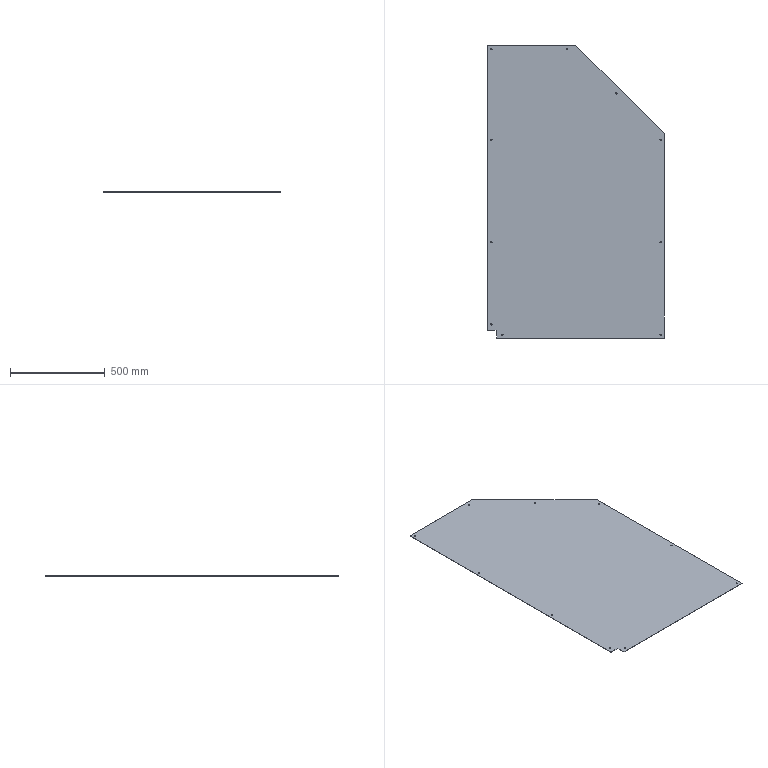Part | SolidWorks | features ICE 5, Fillet 3, HoleWzd 2, Cut 1, FlatPattern 1, SMBaseFlange 1, SheetMetal 1 | 1 solid | 36 faces | box 933 x 1547 x 1.2 mm | volume 1597584 mm3 | cylinder 27 | plane 9 | commonest cylinder face diameters 7 x20 6 x7
STEP:
#1=CARTESIAN_POINT('',(3476.5,-498.,0.));
#2=VERTEX_POINT('',#1);
#3=CARTESIAN_POINT('',(3483.5,-498.,0.));
#4=VERTEX_POINT('',#3);
#5=CARTESIAN_POINT('',(3480.,-498.,0.));
#6=DIRECTION('',(0.,0.,1.));
#7=DIRECTION('',(1.,0.,0.));
#8=AXIS2_PLACEMENT_3D('',#5,#6,#7);
#9=CIRCLE('',#8,3.5);
#10=EDGE_CURVE('',#2,#4,#9,.T.);
#11=ORIENTED_EDGE('',*,*,#10,.F.);
#12=CARTESIAN_POINT('',(3476.5,-498.,1.2));
#13=VERTEX_POINT('',#12);
#14=CARTESIAN_POINT('',(3476.5,-498.,1.2));
#15=DIRECTION('',(0.,0.,1.));
#16=VECTOR('',#15,1000.);
#17=LINE('',#14,#16);
#18=EDGE_CURVE('',#2,#13,#17,.T.);
#19=ORIENTED_EDGE('',*,*,#18,.T.);
#20=CARTESIAN_POINT('',(3483.5,-498.,1.2));
#21=VERTEX_POINT('',#20);
#22=CARTESIAN_POINT('',(3480.,-498.,1.2));
#23=DIRECTION('',(0.,0.,1.));
#24=DIRECTION('',(1.,0.,0.));
#25=AXIS2_PLACEMENT_3D('',#22,#23,#24);
#26=CIRCLE('',#25,3.5);
#27=EDGE_CURVE('',#13,#21,#26,.T.);
#28=ORIENTED_EDGE('',*,*,#27,.T.);
#29=CARTESIAN_POINT('',(3483.5,-498.,1.2));
#30=DIRECTION('',(0.,0.,1.));
#31=VECTOR('',#30,1000.);
#32=LINE('',#29,#31);
#33=EDGE_CURVE('',#4,#21,#32,.T.);
#34=ORIENTED_EDGE('',*,*,#33,.F.);
#35=EDGE_LOOP('',(#11,#19,#28,#34));
#36=FACE_OUTER_BOUND('',#35,.T.);
#37=CARTESIAN_POINT('',(3480.,-498.,1.2));
#38=DIRECTION('',(0.,0.,1.));
#39=DIRECTION('',(1.,0.,0.));
#40=AXIS2_PLACEMENT_3D('',#37,#38,#39);
#41=CYLINDRICAL_SURFACE('',#40,3.5);
#42=ADVANCED_FACE('',(#36),#41,.F.);
#43=CARTESIAN_POINT('',(2583.5,-498.,0.));
#44=VERTEX_POINT('',#43);
#45=CARTESIAN_POINT('',(2590.5,-498.,0.));
#46=VERTEX_POINT('',#45);
#47=CARTESIAN_POINT('',(2587.,-498.,0.));
#48=DIRECTION('',(0.,0.,1.));
#49=DIRECTION('',(1.,0.,0.));
#50=AXIS2_PLACEMENT_3D('',#47,#48,#49);
#51=CIRCLE('',#50,3.5);
#52=EDGE_CURVE('',#44,#46,#51,.T.);
#53=ORIENTED_EDGE('',*,*,#52,.F.);
#54=CARTESIAN_POINT('',(2583.5,-498.,1.2));
#55=VERTEX_POINT('',#54);
#56=CARTESIAN_POINT('',(2583.5,-498.,1.2));
#57=DIRECTION('',(0.,0.,1.));
#58=VECTOR('',#57,1000.);
#59=LINE('',#56,#58);
#60=EDGE_CURVE('',#44,#55,#59,.T.);
#61=ORIENTED_EDGE('',*,*,#60,.T.);
#62=CARTESIAN_POINT('',(2590.5,-498.,1.2));
#63=VERTEX_POINT('',#62);
#64=CARTESIAN_POINT('',(2587.,-498.,1.2));
#65=DIRECTION('',(0.,0.,1.));
#66=DIRECTION('',(1.,0.,0.));
#67=AXIS2_PLACEMENT_3D('',#64,#65,#66);
#68=CIRCLE('',#67,3.5);
#69=EDGE_CURVE('',#55,#63,#68,.T.);
#70=ORIENTED_EDGE('',*,*,#69,.T.);
#71=CARTESIAN_POINT('',(2590.5,-498.,1.2));
#72=DIRECTION('',(0.,0.,1.));
#73=VECTOR('',#72,1000.);
#74=LINE('',#71,#73);
#75=EDGE_CURVE('',#46,#63,#74,.T.);
#76=ORIENTED_EDGE('',*,*,#75,.F.);
#77=EDGE_LOOP('',(#53,#61,#70,#76));
#78=FACE_OUTER_BOUND('',#77,.T.);
#79=CARTESIAN_POINT('',(2587.,-498.,1.2));
#80=DIRECTION('',(0.,0.,1.));
#81=DIRECTION('',(1.,0.,0.));
#82=AXIS2_PLACEMENT_3D('',#79,#80,#81);
#83=CYLINDRICAL_SURFACE('',#82,3.5);
#84=ADVANCED_FACE('',(#78),#83,.F.);
#85=CARTESIAN_POINT('',(2583.5,-20.,0.));
#86=VERTEX_POINT('',#85);
#87=CARTESIAN_POINT('',(2590.5,-20.,0.));
#88=VERTEX_POINT('',#87);
#89=CARTESIAN_POINT('',(2587.,-20.,0.));
#90=DIRECTION('',(0.,0.,1.));
#91=DIRECTION('',(1.,0.,0.));
#92=AXIS2_PLACEMENT_3D('',#89,#90,#91);
#93=CIRCLE('',#92,3.5);
#94=EDGE_CURVE('',#86,#88,#93,.T.);
#95=ORIENTED_EDGE('',*,*,#94,.F.);
#96=CARTESIAN_POINT('',(2583.5,-20.,1.2));
#97=VERTEX_POINT('',#96);
#98=CARTESIAN_POINT('',(2583.5,-20.,1.2));
#99=DIRECTION('',(0.,0.,1.));
#100=VECTOR('',#99,1000.);
#101=LINE('',#98,#100);
#102=EDGE_CURVE('',#86,#97,#101,.T.);
#103=ORIENTED_EDGE('',*,*,#102,.T.);
#104=CARTESIAN_POINT('',(2590.5,-20.,1.2));
#105=VERTEX_POINT('',#104);
#106=CARTESIAN_POINT('',(2587.,-20.,1.2));
#107=DIRECTION('',(0.,0.,1.));
#108=DIRECTION('',(1.,0.,0.));
#109=AXIS2_PLACEMENT_3D('',#106,#107,#108);
#110=CIRCLE('',#109,3.5);
#111=EDGE_CURVE('',#97,#105,#110,.T.);
#112=ORIENTED_EDGE('',*,*,#111,.T.);
#113=CARTESIAN_POINT('',(2590.5,-20.,1.2));
#114=DIRECTION('',(0.,0.,1.));
#115=VECTOR('',#114,1000.);
#116=LINE('',#113,#115);
#117=EDGE_CURVE('',#88,#105,#116,.T.);
#118=ORIENTED_EDGE('',*,*,#117,.F.);
#119=EDGE_LOOP('',(#95,#103,#112,#118));
#120=FACE_OUTER_BOUND('',#119,.T.);
#121=CARTESIAN_POINT('',(2587.,-20.,1.2));
#122=DIRECTION('',(0.,0.,1.));
#123=DIRECTION('',(1.,0.,0.));
#124=AXIS2_PLACEMENT_3D('',#121,#122,#123);
#125=CYLINDRICAL_SURFACE('',#124,3.5);
#126=ADVANCED_FACE('',(#120),#125,.F.);
#127=CARTESIAN_POINT('',(2983.5,-20.,0.));
#128=VERTEX_POINT('',#127);
#129=CARTESIAN_POINT('',(2990.5,-20.,0.));
#130=VERTEX_POINT('',#129);
#131=CARTESIAN_POINT('',(2987.,-20.,0.));
#132=DIRECTION('',(0.,0.,1.));
#133=DIRECTION('',(1.,0.,0.));
#134=AXIS2_PLACEMENT_3D('',#131,#132,#133);
#135=CIRCLE('',#134,3.5);
#136=EDGE_CURVE('',#128,#130,#135,.T.);
#137=ORIENTED_EDGE('',*,*,#136,.F.);
#138=CARTESIAN_POINT('',(2983.5,-20.,1.2));
#139=VERTEX_POINT('',#138);
#140=CARTESIAN_POINT('',(2983.5,-20.,1.2));
#141=DIRECTION('',(0.,0.,1.));
#142=VECTOR('',#141,1000.);
#143=LINE('',#140,#142);
#144=EDGE_CURVE('',#128,#139,#143,.T.);
#145=ORIENTED_EDGE('',*,*,#144,.T.);
#146=CARTESIAN_POINT('',(2990.5,-20.,1.2));
#147=VERTEX_POINT('',#146);
#148=CARTESIAN_POINT('',(2987.,-20.,1.2));
#149=DIRECTION('',(0.,0.,1.));
#150=DIRECTION('',(1.,0.,0.));
#151=AXIS2_PLACEMENT_3D('',#148,#149,#150);
#152=CIRCLE('',#151,3.5);
#153=EDGE_CURVE('',#139,#147,#152,.T.);
#154=ORIENTED_EDGE('',*,*,#153,.T.);
#155=CARTESIAN_POINT('',(2990.5,-20.,1.2));
#156=DIRECTION('',(0.,0.,1.));
#157=VECTOR('',#156,1000.);
#158=LINE('',#155,#157);
#159=EDGE_CURVE('',#130,#147,#158,.T.);
#160=ORIENTED_EDGE('',*,*,#159,.F.);
#161=EDGE_LOOP('',(#137,#145,#154,#160));
#162=FACE_OUTER_BOUND('',#161,.T.);
#163=CARTESIAN_POINT('',(2987.,-20.,1.2));
#164=DIRECTION('',(0.,0.,1.));
#165=DIRECTION('',(1.,0.,0.));
#166=AXIS2_PLACEMENT_3D('',#163,#164,#165);
#167=CYLINDRICAL_SURFACE('',#166,3.5);
#168=ADVANCED_FACE('',(#162),#167,.F.);
#169=CARTESIAN_POINT('',(3476.5,-1039.,0.));
#170=VERTEX_POINT('',#169);
#171=CARTESIAN_POINT('',(3483.5,-1039.,0.));
#172=VERTEX_POINT('',#171);
#173=CARTESIAN_POINT('',(3480.,-1039.,0.));
#174=DIRECTION('',(0.,0.,1.));
#175=DIRECTION('',(1.,0.,0.));
#176=AXIS2_PLACEMENT_3D('',#173,#174,#175);
#177=CIRCLE('',#176,3.5);
#178=EDGE_CURVE('',#170,#172,#177,.T.);
#179=ORIENTED_EDGE('',*,*,#178,.F.);
#180=CARTESIAN_POINT('',(3476.5,-1039.,1.2));
#181=VERTEX_POINT('',#180);
#182=CARTESIAN_POINT('',(3476.5,-1039.,1.2));
#183=DIRECTION('',(0.,0.,1.));
#184=VECTOR('',#183,1000.);
#185=LINE('',#182,#184);
#186=EDGE_CURVE('',#170,#181,#185,.T.);
#187=ORIENTED_EDGE('',*,*,#186,.T.);
#188=CARTESIAN_POINT('',(3483.5,-1039.,1.2));
#189=VERTEX_POINT('',#188);
#190=CARTESIAN_POINT('',(3480.,-1039.,1.2));
#191=DIRECTION('',(0.,0.,1.));
#192=DIRECTION('',(1.,0.,0.));
#193=AXIS2_PLACEMENT_3D('',#190,#191,#192);
#194=CIRCLE('',#193,3.5);
#195=EDGE_CURVE('',#181,#189,#194,.T.);
#196=ORIENTED_EDGE('',*,*,#195,.T.);
#197=CARTESIAN_POINT('',(3483.5,-1039.,1.2));
#198=DIRECTION('',(0.,0.,1.));
#199=VECTOR('',#198,1000.);
#200=LINE('',#197,#199);
#201=EDGE_CURVE('',#172,#189,#200,.T.);
#202=ORIENTED_EDGE('',*,*,#201,.F.);
#203=EDGE_LOOP('',(#179,#187,#196,#202));
#204=FACE_OUTER_BOUND('',#203,.T.);
#205=CARTESIAN_POINT('',(3480.,-1039.,1.2));
#206=DIRECTION('',(0.,0.,1.));
#207=DIRECTION('',(1.,0.,0.));
#208=AXIS2_PLACEMENT_3D('',#205,#206,#207);
#209=CYLINDRICAL_SURFACE('',#208,3.5);
#210=ADVANCED_FACE('',(#204),#209,.F.);
#211=CARTESIAN_POINT('',(3476.5,-1527.,0.));
#212=VERTEX_POINT('',#211);
#213=CARTESIAN_POINT('',(3483.5,-1527.,0.));
#214=VERTEX_POINT('',#213);
#215=CARTESIAN_POINT('',(3480.,-1527.,0.));
#216=DIRECTION('',(0.,0.,1.));
#217=DIRECTION('',(1.,0.,0.));
#218=AXIS2_PLACEMENT_3D('',#215,#216,#217);
#219=CIRCLE('',#218,3.5);
#220=EDGE_CURVE('',#212,#214,#219,.T.);
#221=ORIENTED_EDGE('',*,*,#220,.F.);
#222=CARTESIAN_POINT('',(3476.5,-1527.,1.2));
#223=VERTEX_POINT('',#222);
#224=CARTESIAN_POINT('',(3476.5,-1527.,1.2));
#225=DIRECTION('',(0.,0.,1.));
#226=VECTOR('',#225,1000.);
#227=LINE('',#224,#226);
#228=EDGE_CURVE('',#212,#223,#227,.T.);
#229=ORIENTED_EDGE('',*,*,#228,.T.);
#230=CARTESIAN_POINT('',(3483.5,-1527.,1.2));
#231=VERTEX_POINT('',#230);
#232=CARTESIAN_POINT('',(3480.,-1527.,1.2));
#233=DIRECTION('',(0.,0.,1.));
#234=DIRECTION('',(1.,0.,0.));
#235=AXIS2_PLACEMENT_3D('',#232,#233,#234);
#236=CIRCLE('',#235,3.5);
#237=EDGE_CURVE('',#223,#231,#236,.T.);
#238=ORIENTED_EDGE('',*,*,#237,.T.);
#239=CARTESIAN_POINT('',(3483.5,-1527.,1.2));
#240=DIRECTION('',(0.,0.,1.));
#241=VECTOR('',#240,1000.);
#242=LINE('',#239,#241);
#243=EDGE_CURVE('',#214,#231,#242,.T.);
#244=ORIENTED_EDGE('',*,*,#243,.F.);
#245=EDGE_LOOP('',(#221,#229,#238,#244));
#246=FACE_OUTER_BOUND('',#245,.T.);
#247=CARTESIAN_POINT('',(3480.,-1527.,1.2));
#248=DIRECTION('',(0.,0.,1.));
#249=DIRECTION('',(1.,0.,0.));
#250=AXIS2_PLACEMENT_3D('',#247,#248,#249);
#251=CYLINDRICAL_SURFACE('',#250,3.5);
#252=ADVANCED_FACE('',(#246),#251,.F.);
#253=CARTESIAN_POINT('',(2641.5,-1527.,0.));
#254=VERTEX_POINT('',#253);
#255=CARTESIAN_POINT('',(2648.5,-1527.,0.));
#256=VERTEX_POINT('',#255);
#257=CARTESIAN_POINT('',(2645.,-1527.,0.));
#258=DIRECTION('',(0.,0.,1.));
#259=DIRECTION('',(1.,0.,0.));
#260=AXIS2_PLACEMENT_3D('',#257,#258,#259);
#261=CIRCLE('',#260,3.5);
#262=EDGE_CURVE('',#254,#256,#261,.T.);
#263=ORIENTED_EDGE('',*,*,#262,.F.);
#264=CARTESIAN_POINT('',(2641.5,-1527.,1.2));
#265=VERTEX_POINT('',#264);
#266=CARTESIAN_POINT('',(2641.5,-1527.,1.2));
#267=DIRECTION('',(0.,0.,1.));
#268=VECTOR('',#267,1000.);
#269=LINE('',#266,#268);
#270=EDGE_CURVE('',#254,#265,#269,.T.);
#271=ORIENTED_EDGE('',*,*,#270,.T.);
#272=CARTESIAN_POINT('',(2648.5,-1527.,1.2));
#273=VERTEX_POINT('',#272);
#274=CARTESIAN_POINT('',(2645.,-1527.,1.2));
#275=DIRECTION('',(0.,0.,1.));
#276=DIRECTION('',(1.,0.,0.));
#277=AXIS2_PLACEMENT_3D('',#274,#275,#276);
#278=CIRCLE('',#277,3.5);
#279=EDGE_CURVE('',#265,#273,#278,.T.);
#280=ORIENTED_EDGE('',*,*,#279,.T.);
#281=CARTESIAN_POINT('',(2648.5,-1527.,1.2));
#282=DIRECTION('',(0.,0.,1.));
#283=VECTOR('',#282,1000.);
#284=LINE('',#281,#283);
#285=EDGE_CURVE('',#256,#273,#284,.T.);
#286=ORIENTED_EDGE('',*,*,#285,.F.);
#287=EDGE_LOOP('',(#263,#271,#280,#286));
#288=FACE_OUTER_BOUND('',#287,.T.);
#289=CARTESIAN_POINT('',(2645.,-1527.,1.2));
#290=DIRECTION('',(0.,0.,1.));
#291=DIRECTION('',(1.,0.,0.));
#292=AXIS2_PLACEMENT_3D('',#289,#290,#291);
#293=CYLINDRICAL_SURFACE('',#292,3.5);
#294=ADVANCED_FACE('',(#288),#293,.F.);
#295=CARTESIAN_POINT('',(2583.5,-1472.,0.));
#296=VERTEX_POINT('',#295);
#297=CARTESIAN_POINT('',(2590.5,-1472.,0.));
#298=VERTEX_POINT('',#297);
#299=CARTESIAN_POINT('',(2587.,-1472.,0.));
#300=DIRECTION('',(0.,0.,1.));
#301=DIRECTION('',(1.,0.,0.));
#302=AXIS2_PLACEMENT_3D('',#299,#300,#301);
#303=CIRCLE('',#302,3.5);
#304=EDGE_CURVE('',#296,#298,#303,.T.);
#305=ORIENTED_EDGE('',*,*,#304,.F.);
#306=CARTESIAN_POINT('',(2583.5,-1472.,1.2));
#307=VERTEX_POINT('',#306);
#308=CARTESIAN_POINT('',(2583.5,-1472.,1.2));
#309=DIRECTION('',(0.,0.,1.));
#310=VECTOR('',#309,1000.);
#311=LINE('',#308,#310);
#312=EDGE_CURVE('',#296,#307,#311,.T.);
#313=ORIENTED_EDGE('',*,*,#312,.T.);
#314=CARTESIAN_POINT('',(2590.5,-1472.,1.2));
#315=VERTEX_POINT('',#314);
#316=CARTESIAN_POINT('',(2587.,-1472.,1.2));
#317=DIRECTION('',(0.,0.,1.));
#318=DIRECTION('',(1.,0.,0.));
#319=AXIS2_PLACEMENT_3D('',#316,#317,#318);
#320=CIRCLE('',#319,3.5);
#321=EDGE_CURVE('',#307,#315,#320,.T.);
#322=ORIENTED_EDGE('',*,*,#321,.T.);
#323=CARTESIAN_POINT('',(2590.5,-1472.,1.2));
#324=DIRECTION('',(0.,0.,1.));
#325=VECTOR('',#324,1000.);
#326=LINE('',#323,#325);
#327=EDGE_CURVE('',#298,#315,#326,.T.);
#328=ORIENTED_EDGE('',*,*,#327,.F.);
#329=EDGE_LOOP('',(#305,#313,#322,#328));
#330=FACE_OUTER_BOUND('',#329,.T.);
#331=CARTESIAN_POINT('',(2587.,-1472.,1.2));
#332=DIRECTION('',(0.,0.,1.));
#333=DIRECTION('',(1.,0.,0.));
#334=AXIS2_PLACEMENT_3D('',#331,#332,#333);
#335=CYLINDRICAL_SURFACE('',#334,3.5);
#336=ADVANCED_FACE('',(#330),#335,.F.);
#337=CARTESIAN_POINT('',(3243.074,-253.426,0.));
#338=VERTEX_POINT('',#337);
#339=CARTESIAN_POINT('',(3250.074,-253.426,0.));
#340=VERTEX_POINT('',#339);
#341=CARTESIAN_POINT('',(3246.574,-253.426,0.));
#342=DIRECTION('',(0.,0.,1.));
#343=DIRECTION('',(1.,0.,0.));
#344=AXIS2_PLACEMENT_3D('',#341,#342,#343);
#345=CIRCLE('',#344,3.5);
#346=EDGE_CURVE('',#338,#340,#345,.T.);
#347=ORIENTED_EDGE('',*,*,#346,.F.);
#348=CARTESIAN_POINT('',(3243.074,-253.426,1.2));
#349=VERTEX_POINT('',#348);
#350=CARTESIAN_POINT('',(3243.074,-253.426,1.2));
#351=DIRECTION('',(0.,0.,1.));
#352=VECTOR('',#351,1000.);
#353=LINE('',#350,#352);
#354=EDGE_CURVE('',#338,#349,#353,.T.);
#355=ORIENTED_EDGE('',*,*,#354,.T.);
#356=CARTESIAN_POINT('',(3250.074,-253.426,1.2));
#357=VERTEX_POINT('',#356);
#358=CARTESIAN_POINT('',(3246.574,-253.426,1.2));
#359=DIRECTION('',(0.,0.,1.));
#360=DIRECTION('',(1.,0.,0.));
#361=AXIS2_PLACEMENT_3D('',#358,#359,#360);
#362=CIRCLE('',#361,3.5);
#363=EDGE_CURVE('',#349,#357,#362,.T.);
#364=ORIENTED_EDGE('',*,*,#363,.T.);
#365=CARTESIAN_POINT('',(3250.074,-253.426,1.2));
#366=DIRECTION('',(0.,0.,1.));
#367=VECTOR('',#366,1000.);
#368=LINE('',#365,#367);
#369=EDGE_CURVE('',#340,#357,#368,.T.);
#370=ORIENTED_EDGE('',*,*,#369,.F.);
#371=EDGE_LOOP('',(#347,#355,#364,#370));
#372=FACE_OUTER_BOUND('',#371,.T.);
#373=CARTESIAN_POINT('',(3246.574,-253.426,1.2));
#374=DIRECTION('',(0.,0.,1.));
#375=DIRECTION('',(1.,0.,0.));
#376=AXIS2_PLACEMENT_3D('',#373,#374,#375);
#377=CYLINDRICAL_SURFACE('',#376,3.5);
#378=ADVANCED_FACE('',(#372),#377,.F.);
#379=CARTESIAN_POINT('',(2583.5,-1039.,0.));
#380=VERTEX_POINT('',#379);
#381=CARTESIAN_POINT('',(2590.5,-1039.,0.));
#382=VERTEX_POINT('',#381);
#383=CARTESIAN_POINT('',(2587.,-1039.,0.));
#384=DIRECTION('',(0.,0.,1.));
#385=DIRECTION('',(1.,0.,0.));
#386=AXIS2_PLACEMENT_3D('',#383,#384,#385);
#387=CIRCLE('',#386,3.5);
#388=EDGE_CURVE('',#380,#382,#387,.T.);
#389=ORIENTED_EDGE('',*,*,#388,.F.);
#390=CARTESIAN_POINT('',(2583.5,-1039.,1.2));
#391=VERTEX_POINT('',#390);
#392=CARTESIAN_POINT('',(2583.5,-1039.,1.2));
#393=DIRECTION('',(0.,0.,1.));
#394=VECTOR('',#393,1000.);
#395=LINE('',#392,#394);
#396=EDGE_CURVE('',#380,#391,#395,.T.);
#397=ORIENTED_EDGE('',*,*,#396,.T.);
#398=CARTESIAN_POINT('',(2590.5,-1039.,1.2));
#399=VERTEX_POINT('',#398);
#400=CARTESIAN_POINT('',(2587.,-1039.,1.2));
#401=DIRECTION('',(0.,0.,1.));
#402=DIRECTION('',(1.,0.,0.));
#403=AXIS2_PLACEMENT_3D('',#400,#401,#402);
#404=CIRCLE('',#403,3.5);
#405=EDGE_CURVE('',#391,#399,#404,.T.);
#406=ORIENTED_EDGE('',*,*,#405,.T.);
#407=CARTESIAN_POINT('',(2590.5,-1039.,1.2));
#408=DIRECTION('',(0.,0.,1.));
#409=VECTOR('',#408,1000.);
#410=LINE('',#407,#409);
#411=EDGE_CURVE('',#382,#399,#410,.T.);
#412=ORIENTED_EDGE('',*,*,#411,.F.);
#413=EDGE_LOOP('',(#389,#397,#406,#412));
#414=FACE_OUTER_BOUND('',#413,.T.);
#415=CARTESIAN_POINT('',(2587.,-1039.,1.2));
#416=DIRECTION('',(0.,0.,1.));
#417=DIRECTION('',(1.,0.,0.));
#418=AXIS2_PLACEMENT_3D('',#415,#416,#417);
#419=CYLINDRICAL_SURFACE('',#418,3.5);
#420=ADVANCED_FACE('',(#414),#419,.F.);
#421=CARTESIAN_POINT('',(3497.,-1547.,1.2));
#422=VERTEX_POINT('',#421);
#423=CARTESIAN_POINT('',(2618.,-1547.,1.2));
#424=VERTEX_POINT('',#423);
#425=CARTESIAN_POINT('',(0.,-1547.,1.2));
#426=DIRECTION('',(-1.,0.,0.));
#427=VECTOR('',#426,1000.);
#428=LINE('',#425,#427);
#429=EDGE_CURVE('',#422,#424,#428,.T.);
#430=ORIENTED_EDGE('',*,*,#429,.T.);
#431=CARTESIAN_POINT('',(2618.,-1547.,0.));
#432=VERTEX_POINT('',#431);
#433=CARTESIAN_POINT('',(2618.,-1547.,0.));
#434=DIRECTION('',(0.,0.,-1.));
#435=VECTOR('',#434,1000.);
#436=LINE('',#433,#435);
#437=EDGE_CURVE('',#424,#432,#436,.T.);
#438=ORIENTED_EDGE('',*,*,#437,.T.);
#439=CARTESIAN_POINT('',(3497.,-1547.,0.));
#440=VERTEX_POINT('',#439);
#441=CARTESIAN_POINT('',(0.,-1547.,0.));
#442=DIRECTION('',(-1.,0.,0.));
#443=VECTOR('',#442,1000.);
#444=LINE('',#441,#443);
#445=EDGE_CURVE('',#440,#432,#444,.T.);
#446=ORIENTED_EDGE('',*,*,#445,.F.);
#447=CARTESIAN_POINT('',(3497.,-1547.,1.2));
#448=DIRECTION('',(0.,0.,1.));
#449=VECTOR('',#448,1000.);
#450=LINE('',#447,#449);
#451=EDGE_CURVE('',#440,#422,#450,.T.);
#452=ORIENTED_EDGE('',*,*,#451,.T.);
#453=EDGE_LOOP('',(#430,#438,#446,#452));
#454=FACE_OUTER_BOUND('',#453,.T.);
#455=CARTESIAN_POINT('',(0.,-1547.,1.2));
#456=DIRECTION('',(0.,-1.,0.));
#457=DIRECTION('',(0.,0.,-1.));
#458=AXIS2_PLACEMENT_3D('',#455,#456,#457);
#459=PLANE('',#458);
#460=ADVANCED_FACE('',(#454),#459,.T.);
#461=CARTESIAN_POINT('',(3500.,-469.174,0.));
#462=VERTEX_POINT('',#461);
#463=CARTESIAN_POINT('',(3500.,-1544.,0.));
#464=VERTEX_POINT('',#463);
#465=CARTESIAN_POINT('',(3500.,0.,0.));
#466=DIRECTION('',(0.,-1.,0.));
#467=VECTOR('',#466,1000.);
#468=LINE('',#465,#467);
#469=EDGE_CURVE('',#462,#464,#468,.T.);
#470=ORIENTED_EDGE('',*,*,#469,.F.);
#471=CARTESIAN_POINT('',(3500.,-469.174,1.2));
#472=VERTEX_POINT('',#471);
#473=CARTESIAN_POINT('',(3500.,-469.174,1.2));
#474=DIRECTION('',(0.,0.,1.));
#475=VECTOR('',#474,1000.);
#476=LINE('',#473,#475);
#477=EDGE_CURVE('',#462,#472,#476,.T.);
#478=ORIENTED_EDGE('',*,*,#477,.T.);
#479=CARTESIAN_POINT('',(3500.,-1544.,1.2));
#480=VERTEX_POINT('',#479);
#481=CARTESIAN_POINT('',(3500.,0.,1.2));
#482=DIRECTION('',(0.,-1.,0.));
#483=VECTOR('',#482,1000.);
#484=LINE('',#481,#483);
#485=EDGE_CURVE('',#472,#480,#484,.T.);
#486=ORIENTED_EDGE('',*,*,#485,.T.);
#487=CARTESIAN_POINT('',(3500.,-1544.,1.2));
#488=DIRECTION('',(0.,0.,-1.));
#489=VECTOR('',#488,1000.);
#490=LINE('',#487,#489);
#491=EDGE_CURVE('',#480,#464,#490,.T.);
#492=ORIENTED_EDGE('',*,*,#491,.T.);
#493=EDGE_LOOP('',(#470,#478,#486,#492));
#494=FACE_OUTER_BOUND('',#493,.T.);
#495=CARTESIAN_POINT('',(3500.,0.,1.2));
#496=DIRECTION('',(1.,0.,0.));
#497=DIRECTION('',(0.,0.,-1.));
#498=AXIS2_PLACEMENT_3D('',#495,#496,#497);
#499=PLANE('',#498);
#500=ADVANCED_FACE('',(#494),#499,.T.);
#501=CARTESIAN_POINT('',(2615.,-1544.,1.2));
#502=VERTEX_POINT('',#501);
#503=CARTESIAN_POINT('',(2615.,-1505.,1.2));
#504=VERTEX_POINT('',#503);
#505=CARTESIAN_POINT('',(2615.,-1547.,1.2));
#506=DIRECTION('',(0.,1.,0.));
#507=VECTOR('',#506,1000.);
#508=LINE('',#505,#507);
#509=EDGE_CURVE('',#502,#504,#508,.T.);
#510=ORIENTED_EDGE('',*,*,#509,.T.);
#511=CARTESIAN_POINT('',(2615.,-1505.,0.));
#512=VERTEX_POINT('',#511);
#513=CARTESIAN_POINT('',(2615.,-1505.,0.));
#514=DIRECTION('',(0.,0.,-1.));
#515=VECTOR('',#514,1000.);
#516=LINE('',#513,#515);
#517=EDGE_CURVE('',#504,#512,#516,.T.);
#518=ORIENTED_EDGE('',*,*,#517,.T.);
#519=CARTESIAN_POINT('',(2615.,-1544.,0.));
#520=VERTEX_POINT('',#519);
#521=CARTESIAN_POINT('',(2615.,0.,0.));
#522=DIRECTION('',(0.,1.,0.));
#523=VECTOR('',#522,1000.);
#524=LINE('',#521,#523);
#525=EDGE_CURVE('',#520,#512,#524,.T.);
#526=ORIENTED_EDGE('',*,*,#525,.F.);
#527=CARTESIAN_POINT('',(2615.,-1544.,1.2));
#528=DIRECTION('',(0.,0.,1.));
#529=VECTOR('',#528,1000.);
#530=LINE('',#527,#529);
#531=EDGE_CURVE('',#520,#502,#530,.T.);
#532=ORIENTED_EDGE('',*,*,#531,.T.);
#533=EDGE_LOOP('',(#510,#518,#526,#532));
#534=FACE_OUTER_BOUND('',#533,.T.);
#535=CARTESIAN_POINT('',(2615.,-1547.,-8.8));
#536=DIRECTION('',(1.,0.,0.));
#537=DIRECTION('',(0.,0.,-1.));
#538=AXIS2_PLACEMENT_3D('',#535,#536,#537);
#539=PLANE('',#538);
#540=ADVANCED_FACE('',(#534),#539,.F.);
#541=CARTESIAN_POINT('',(2612.,-1502.,1.2));
#542=VERTEX_POINT('',#541);
#543=CARTESIAN_POINT('',(2570.,-1502.,1.2));
#544=VERTEX_POINT('',#543);
#545=CARTESIAN_POINT('',(885.,-1502.,1.2));
#546=DIRECTION('',(-1.,0.,0.));
#547=VECTOR('',#546,1000.);
#548=LINE('',#545,#547);
#549=EDGE_CURVE('',#542,#544,#548,.T.);
#550=ORIENTED_EDGE('',*,*,#549,.T.);
#551=CARTESIAN_POINT('',(2570.,-1502.,0.));
#552=VERTEX_POINT('',#551);
#553=CARTESIAN_POINT('',(2570.,-1502.,-8.8));
#554=DIRECTION('',(0.,0.,-1.));
#555=VECTOR('',#554,1000.);
#556=LINE('',#553,#555);
#557=EDGE_CURVE('',#544,#552,#556,.T.);
#558=ORIENTED_EDGE('',*,*,#557,.T.);
#559=CARTESIAN_POINT('',(2612.,-1502.,0.));
#560=VERTEX_POINT('',#559);
#561=CARTESIAN_POINT('',(0.,-1502.,0.));
#562=DIRECTION('',(-1.,0.,0.));
#563=VECTOR('',#562,1000.);
#564=LINE('',#561,#563);
#565=EDGE_CURVE('',#560,#552,#564,.T.);
#566=ORIENTED_EDGE('',*,*,#565,.F.);
#567=CARTESIAN_POINT('',(2612.,-1502.,1.2));
#568=DIRECTION('',(0.,0.,1.));
#569=VECTOR('',#568,1000.);
#570=LINE('',#567,#569);
#571=EDGE_CURVE('',#560,#542,#570,.T.);
#572=ORIENTED_EDGE('',*,*,#571,.T.);
#573=EDGE_LOOP('',(#550,#558,#566,#572));
#574=FACE_OUTER_BOUND('',#573,.T.);
#575=CARTESIAN_POINT('',(885.,-1502.,-8.8));
#576=DIRECTION('',(0.,1.,0.));
#577=DIRECTION('',(0.,0.,1.));
#578=AXIS2_PLACEMENT_3D('',#575,#576,#577);
#579=PLANE('',#578);
#580=ADVANCED_FACE('',(#574),#579,.F.);
#581=CARTESIAN_POINT('',(3480.,-498.,0.));
#582=DIRECTION('',(0.,0.,1.));
#583=DIRECTION('',(1.,0.,0.));
#584=AXIS2_PLACEMENT_3D('',#581,#582,#583);
#585=CIRCLE('',#584,3.5);
#586=EDGE_CURVE('',#4,#2,#585,.T.);
#587=ORIENTED_EDGE('',*,*,#586,.T.);
#588=ORIENTED_EDGE('',*,*,#10,.T.);
#589=EDGE_LOOP('',(#587,#588));
#590=FACE_BOUND('',#589,.T.);
#591=CARTESIAN_POINT('',(2587.,-498.,0.));
#592=DIRECTION('',(0.,0.,1.));
#593=DIRECTION('',(1.,0.,0.));
#594=AXIS2_PLACEMENT_3D('',#591,#592,#593);
#595=CIRCLE('',#594,3.5);
#596=EDGE_CURVE('',#46,#44,#595,.T.);
#597=ORIENTED_EDGE('',*,*,#596,.T.);
#598=ORIENTED_EDGE('',*,*,#52,.T.);
#599=EDGE_LOOP('',(#597,#598));
#600=FACE_BOUND('',#599,.T.);
#601=CARTESIAN_POINT('',(2587.,-20.,0.));
#602=DIRECTION('',(0.,0.,1.));
#603=DIRECTION('',(1.,0.,0.));
#604=AXIS2_PLACEMENT_3D('',#601,#602,#603);
#605=CIRCLE('',#604,3.5);
#606=EDGE_CURVE('',#88,#86,#605,.T.);
#607=ORIENTED_EDGE('',*,*,#606,.T.);
#608=ORIENTED_EDGE('',*,*,#94,.T.);
#609=EDGE_LOOP('',(#607,#608));
#610=FACE_BOUND('',#609,.T.);
#611=CARTESIAN_POINT('',(2987.,-20.,0.));
#612=DIRECTION('',(0.,0.,1.));
#613=DIRECTION('',(1.,0.,0.));
#614=AXIS2_PLACEMENT_3D('',#611,#612,#613);
#615=CIRCLE('',#614,3.5);
#616=EDGE_CURVE('',#130,#128,#615,.T.);
#617=ORIENTED_EDGE('',*,*,#616,.T.);
#618=ORIENTED_EDGE('',*,*,#136,.T.);
#619=EDGE_LOOP('',(#617,#618));
#620=FACE_BOUND('',#619,.T.);
#621=CARTESIAN_POINT('',(3480.,-1039.,0.));
#622=DIRECTION('',(0.,0.,1.));
#623=DIRECTION('',(1.,0.,0.));
#624=AXIS2_PLACEMENT_3D('',#621,#622,#623);
#625=CIRCLE('',#624,3.5);
#626=EDGE_CURVE('',#172,#170,#625,.T.);
#627=ORIENTED_EDGE('',*,*,#626,.T.);
#628=ORIENTED_EDGE('',*,*,#178,.T.);
#629=EDGE_LOOP('',(#627,#628));
#630=FACE_BOUND('',#629,.T.);
#631=CARTESIAN_POINT('',(3480.,-1527.,0.));
#632=DIRECTION('',(0.,0.,1.));
#633=DIRECTION('',(1.,0.,0.));
#634=AXIS2_PLACEMENT_3D('',#631,#632,#633);
#635=CIRCLE('',#634,3.5);
#636=EDGE_CURVE('',#214,#212,#635,.T.);
#637=ORIENTED_EDGE('',*,*,#636,.T.);
#638=ORIENTED_EDGE('',*,*,#220,.T.);
#639=EDGE_LOOP('',(#637,#638));
#640=FACE_BOUND('',#639,.T.);
#641=CARTESIAN_POINT('',(2645.,-1527.,0.));
#642=DIRECTION('',(0.,0.,1.));
#643=DIRECTION('',(1.,0.,0.));
#644=AXIS2_PLACEMENT_3D('',#641,#642,#643);
#645=CIRCLE('',#644,3.5);
#646=EDGE_CURVE('',#256,#254,#645,.T.);
#647=ORIENTED_EDGE('',*,*,#646,.T.);
#648=ORIENTED_EDGE('',*,*,#262,.T.);
#649=EDGE_LOOP('',(#647,#648));
#650=FACE_BOUND('',#649,.T.);
#651=CARTESIAN_POINT('',(2587.,-1472.,0.));
#652=DIRECTION('',(0.,0.,1.));
#653=DIRECTION('',(1.,0.,0.));
#654=AXIS2_PLACEMENT_3D('',#651,#652,#653);
#655=CIRCLE('',#654,3.5);
#656=EDGE_CURVE('',#298,#296,#655,.T.);
#657=ORIENTED_EDGE('',*,*,#656,.T.);
#658=ORIENTED_EDGE('',*,*,#304,.T.);
#659=EDGE_LOOP('',(#657,#658));
#660=FACE_BOUND('',#659,.T.);
#661=CARTESIAN_POINT('',(3246.574,-253.426,0.));
#662=DIRECTION('',(0.,0.,1.));
#663=DIRECTION('',(1.,0.,0.));
#664=AXIS2_PLACEMENT_3D('',#661,#662,#663);
#665=CIRCLE('',#664,3.5);
#666=EDGE_CURVE('',#340,#338,#665,.T.);
#667=ORIENTED_EDGE('',*,*,#666,.T.);
#668=ORIENTED_EDGE('',*,*,#346,.T.);
#669=EDGE_LOOP('',(#667,#668));
#670=FACE_BOUND('',#669,.T.);
#671=CARTESIAN_POINT('',(2587.,-1039.,0.));
#672=DIRECTION('',(0.,0.,1.));
#673=DIRECTION('',(1.,0.,0.));
#674=AXIS2_PLACEMENT_3D('',#671,#672,#673);
#675=CIRCLE('',#674,3.5);
#676=EDGE_CURVE('',#382,#380,#675,.T.);
#677=ORIENTED_EDGE('',*,*,#676,.T.);
#678=ORIENTED_EDGE('',*,*,#388,.T.);
#679=EDGE_LOOP('',(#677,#678));
#680=FACE_BOUND('',#679,.T.);
#681=CARTESIAN_POINT('',(3499.121,-467.053,0.));
#682=VERTEX_POINT('',#681);
#683=CARTESIAN_POINT('',(3032.947,-0.8787,0.));
#684=VERTEX_POINT('',#683);
#685=CARTESIAN_POINT('',(3511.835,-479.766,0.));
#686=DIRECTION('',(-0.7071,0.7071,0.));
#687=VECTOR('',#686,1000.);
#688=LINE('',#685,#687);
#689=EDGE_CURVE('',#682,#684,#688,.T.);
#690=ORIENTED_EDGE('',*,*,#689,.F.);
#691=CARTESIAN_POINT('',(3497.,-469.174,0.));
#692=DIRECTION('',(0.,0.,-1.));
#693=DIRECTION('',(1.,0.,0.));
#694=AXIS2_PLACEMENT_3D('',#691,#692,#693);
#695=CIRCLE('',#694,3.);
#696=EDGE_CURVE('',#682,#462,#695,.T.);
#697=ORIENTED_EDGE('',*,*,#696,.T.);
#698=ORIENTED_EDGE('',*,*,#469,.T.);
#699=CARTESIAN_POINT('',(3497.,-1544.,0.));
#700=DIRECTION('',(0.,0.,-1.));
#701=DIRECTION('',(1.,0.,0.));
#702=AXIS2_PLACEMENT_3D('',#699,#700,#701);
#703=CIRCLE('',#702,3.);
#704=EDGE_CURVE('',#464,#440,#703,.T.);
#705=ORIENTED_EDGE('',*,*,#704,.T.);
#706=ORIENTED_EDGE('',*,*,#445,.T.);
#707=CARTESIAN_POINT('',(2618.,-1544.,0.));
#708=DIRECTION('',(0.,0.,-1.));
#709=DIRECTION('',(1.,0.,0.));
#710=AXIS2_PLACEMENT_3D('',#707,#708,#709);
#711=CIRCLE('',#710,3.);
#712=EDGE_CURVE('',#432,#520,#711,.T.);
#713=ORIENTED_EDGE('',*,*,#712,.T.);
#714=ORIENTED_EDGE('',*,*,#525,.T.);
#715=CARTESIAN_POINT('',(2612.,-1505.,0.));
#716=DIRECTION('',(0.,0.,1.));
#717=DIRECTION('',(1.,0.,0.));
#718=AXIS2_PLACEMENT_3D('',#715,#716,#717);
#719=CIRCLE('',#718,3.);
#720=EDGE_CURVE('',#512,#560,#719,.T.);
#721=ORIENTED_EDGE('',*,*,#720,.T.);
#722=ORIENTED_EDGE('',*,*,#565,.T.);
#723=CARTESIAN_POINT('',(2567.,-1499.,0.));
#724=VERTEX_POINT('',#723);
#725=CARTESIAN_POINT('',(2570.,-1499.,0.));
#726=DIRECTION('',(0.,0.,-1.));
#727=DIRECTION('',(1.,0.,0.));
#728=AXIS2_PLACEMENT_3D('',#725,#726,#727);
#729=CIRCLE('',#728,3.);
#730=EDGE_CURVE('',#552,#724,#729,.T.);
#731=ORIENTED_EDGE('',*,*,#730,.T.);
#732=CARTESIAN_POINT('',(2567.,-3.,0.));
#733=VERTEX_POINT('',#732);
#734=CARTESIAN_POINT('',(2567.,0.,0.));
#735=DIRECTION('',(0.,1.,0.));
#736=VECTOR('',#735,1000.);
#737=LINE('',#734,#736);
#738=EDGE_CURVE('',#724,#733,#737,.T.);
#739=ORIENTED_EDGE('',*,*,#738,.T.);
#740=CARTESIAN_POINT('',(2570.,0.,0.));
#741=VERTEX_POINT('',#740);
#742=CARTESIAN_POINT('',(2570.,-3.,0.));
#743=DIRECTION('',(0.,0.,-1.));
#744=DIRECTION('',(1.,0.,0.));
#745=AXIS2_PLACEMENT_3D('',#742,#743,#744);
#746=CIRCLE('',#745,3.);
#747=EDGE_CURVE('',#733,#741,#746,.T.);
#748=ORIENTED_EDGE('',*,*,#747,.T.);
#749=CARTESIAN_POINT('',(3030.826,0.,0.));
#750=VERTEX_POINT('',#749);
#751=CARTESIAN_POINT('',(0.,0.,0.));
#752=DIRECTION('',(1.,0.,0.));
#753=VECTOR('',#752,1000.);
#754=LINE('',#751,#753);
#755=EDGE_CURVE('',#741,#750,#754,.T.);
#756=ORIENTED_EDGE('',*,*,#755,.T.);
#757=CARTESIAN_POINT('',(3030.826,-3.,0.));
#758=DIRECTION('',(0.,0.,-1.));
#759=DIRECTION('',(1.,0.,0.));
#760=AXIS2_PLACEMENT_3D('',#757,#758,#759);
#761=CIRCLE('',#760,3.);
#762=EDGE_CURVE('',#750,#684,#761,.T.);
#763=ORIENTED_EDGE('',*,*,#762,.T.);
#764=EDGE_LOOP('',(#690,#697,#698,#705,#706,#713,#714,#721,#722,#731,#739,#748,#756,#763));
#765=FACE_OUTER_BOUND('',#764,.T.);
#766=CARTESIAN_POINT('',(0.,0.,0.));
#767=DIRECTION('',(0.,0.,1.));
#768=DIRECTION('',(1.,0.,0.));
#769=AXIS2_PLACEMENT_3D('',#766,#767,#768);
#770=PLANE('',#769);
#771=ADVANCED_FACE('',(#590,#600,#610,#620,#630,#640,#650,#660,#670,#680,#765),#770,.F.);
#772=ORIENTED_EDGE('',*,*,#485,.F.);
#773=CARTESIAN_POINT('',(3499.121,-467.053,1.2));
#774=VERTEX_POINT('',#773);
#775=CARTESIAN_POINT('',(3497.,-469.174,1.2));
#776=DIRECTION('',(0.,0.,1.));
#777=DIRECTION('',(1.,0.,0.));
#778=AXIS2_PLACEMENT_3D('',#775,#776,#777);
#779=CIRCLE('',#778,3.);
#780=EDGE_CURVE('',#472,#774,#779,.T.);
#781=ORIENTED_EDGE('',*,*,#780,.T.);
#782=CARTESIAN_POINT('',(3032.947,-0.8787,1.2));
#783=VERTEX_POINT('',#782);
#784=CARTESIAN_POINT('',(1516.034,1516.034,1.2));
#785=DIRECTION('',(0.7071,-0.7071,0.));
#786=VECTOR('',#785,1000.);
#787=LINE('',#784,#786);
#788=EDGE_CURVE('',#783,#774,#787,.T.);
#789=ORIENTED_EDGE('',*,*,#788,.F.);
#790=CARTESIAN_POINT('',(3030.826,0.,1.2));
#791=VERTEX_POINT('',#790);
#792=CARTESIAN_POINT('',(3030.826,-3.,1.2));
#793=DIRECTION('',(0.,0.,1.));
#794=DIRECTION('',(1.,0.,0.));
#795=AXIS2_PLACEMENT_3D('',#792,#793,#794);
#796=CIRCLE('',#795,3.);
#797=EDGE_CURVE('',#783,#791,#796,.T.);
#798=ORIENTED_EDGE('',*,*,#797,.T.);
#799=CARTESIAN_POINT('',(2570.,0.,1.2));
#800=VERTEX_POINT('',#799);
#801=CARTESIAN_POINT('',(0.,0.,1.2));
#802=DIRECTION('',(1.,0.,0.));
#803=VECTOR('',#802,1000.);
#804=LINE('',#801,#803);
#805=EDGE_CURVE('',#800,#791,#804,.T.);
#806=ORIENTED_EDGE('',*,*,#805,.F.);
#807=CARTESIAN_POINT('',(2567.,-3.,1.2));
#808=VERTEX_POINT('',#807);
#809=CARTESIAN_POINT('',(2570.,-3.,1.2));
#810=DIRECTION('',(0.,0.,1.));
#811=DIRECTION('',(1.,0.,0.));
#812=AXIS2_PLACEMENT_3D('',#809,#810,#811);
#813=CIRCLE('',#812,3.);
#814=EDGE_CURVE('',#800,#808,#813,.T.);
#815=ORIENTED_EDGE('',*,*,#814,.T.);
#816=CARTESIAN_POINT('',(2567.,-1499.,1.2));
#817=VERTEX_POINT('',#816);
#818=CARTESIAN_POINT('',(2567.,-1651.39,1.2));
#819=DIRECTION('',(0.,1.,0.));
#820=VECTOR('',#819,1000.);
#821=LINE('',#818,#820);
#822=EDGE_CURVE('',#817,#808,#821,.T.);
#823=ORIENTED_EDGE('',*,*,#822,.F.);
#824=CARTESIAN_POINT('',(2570.,-1499.,1.2));
#825=DIRECTION('',(0.,0.,1.));
#826=DIRECTION('',(1.,0.,0.));
#827=AXIS2_PLACEMENT_3D('',#824,#825,#826);
#828=CIRCLE('',#827,3.);
#829=EDGE_CURVE('',#817,#544,#828,.T.);
#830=ORIENTED_EDGE('',*,*,#829,.T.);
#831=ORIENTED_EDGE('',*,*,#549,.F.);
#832=CARTESIAN_POINT('',(2612.,-1505.,1.2));
#833=DIRECTION('',(0.,0.,-1.));
#834=DIRECTION('',(1.,0.,0.));
#835=AXIS2_PLACEMENT_3D('',#832,#833,#834);
#836=CIRCLE('',#835,3.);
#837=EDGE_CURVE('',#542,#504,#836,.T.);
#838=ORIENTED_EDGE('',*,*,#837,.T.);
#839=ORIENTED_EDGE('',*,*,#509,.F.);
#840=CARTESIAN_POINT('',(2618.,-1544.,1.2));
#841=DIRECTION('',(0.,0.,1.));
#842=DIRECTION('',(1.,0.,0.));
#843=AXIS2_PLACEMENT_3D('',#840,#841,#842);
#844=CIRCLE('',#843,3.);
#845=EDGE_CURVE('',#502,#424,#844,.T.);
#846=ORIENTED_EDGE('',*,*,#845,.T.);
#847=ORIENTED_EDGE('',*,*,#429,.F.);
#848=CARTESIAN_POINT('',(3497.,-1544.,1.2));
#849=DIRECTION('',(0.,0.,1.));
#850=DIRECTION('',(1.,0.,0.));
#851=AXIS2_PLACEMENT_3D('',#848,#849,#850);
#852=CIRCLE('',#851,3.);
#853=EDGE_CURVE('',#422,#480,#852,.T.);
#854=ORIENTED_EDGE('',*,*,#853,.T.);
#855=EDGE_LOOP('',(#772,#781,#789,#798,#806,#815,#823,#830,#831,#838,#839,#846,#847,#854));
#856=FACE_OUTER_BOUND('',#855,.T.);
#857=CARTESIAN_POINT('',(3480.,-498.,1.2));
#858=DIRECTION('',(0.,0.,1.));
#859=DIRECTION('',(1.,0.,0.));
#860=AXIS2_PLACEMENT_3D('',#857,#858,#859);
#861=CIRCLE('',#860,3.5);
#862=EDGE_CURVE('',#21,#13,#861,.T.);
#863=ORIENTED_EDGE('',*,*,#862,.F.);
#864=ORIENTED_EDGE('',*,*,#27,.F.);
#865=EDGE_LOOP('',(#863,#864));
#866=FACE_BOUND('',#865,.T.);
#867=CARTESIAN_POINT('',(2587.,-498.,1.2));
#868=DIRECTION('',(0.,0.,1.));
#869=DIRECTION('',(1.,0.,0.));
#870=AXIS2_PLACEMENT_3D('',#867,#868,#869);
#871=CIRCLE('',#870,3.5);
#872=EDGE_CURVE('',#63,#55,#871,.T.);
#873=ORIENTED_EDGE('',*,*,#872,.F.);
#874=ORIENTED_EDGE('',*,*,#69,.F.);
#875=EDGE_LOOP('',(#873,#874));
#876=FACE_BOUND('',#875,.T.);
#877=CARTESIAN_POINT('',(2587.,-20.,1.2));
#878=DIRECTION('',(0.,0.,1.));
#879=DIRECTION('',(1.,0.,0.));
#880=AXIS2_PLACEMENT_3D('',#877,#878,#879);
#881=CIRCLE('',#880,3.5);
#882=EDGE_CURVE('',#105,#97,#881,.T.);
#883=ORIENTED_EDGE('',*,*,#882,.F.);
#884=ORIENTED_EDGE('',*,*,#111,.F.);
#885=EDGE_LOOP('',(#883,#884));
#886=FACE_BOUND('',#885,.T.);
#887=CARTESIAN_POINT('',(2987.,-20.,1.2));
#888=DIRECTION('',(0.,0.,1.));
#889=DIRECTION('',(1.,0.,0.));
#890=AXIS2_PLACEMENT_3D('',#887,#888,#889);
#891=CIRCLE('',#890,3.5);
#892=EDGE_CURVE('',#147,#139,#891,.T.);
#893=ORIENTED_EDGE('',*,*,#892,.F.);
#894=ORIENTED_EDGE('',*,*,#153,.F.);
#895=EDGE_LOOP('',(#893,#894));
#896=FACE_BOUND('',#895,.T.);
#897=CARTESIAN_POINT('',(3480.,-1039.,1.2));
#898=DIRECTION('',(0.,0.,1.));
#899=DIRECTION('',(1.,0.,0.));
#900=AXIS2_PLACEMENT_3D('',#897,#898,#899);
#901=CIRCLE('',#900,3.5);
#902=EDGE_CURVE('',#189,#181,#901,.T.);
#903=ORIENTED_EDGE('',*,*,#902,.F.);
#904=ORIENTED_EDGE('',*,*,#195,.F.);
#905=EDGE_LOOP('',(#903,#904));
#906=FACE_BOUND('',#905,.T.);
#907=CARTESIAN_POINT('',(3480.,-1527.,1.2));
#908=DIRECTION('',(0.,0.,1.));
#909=DIRECTION('',(1.,0.,0.));
#910=AXIS2_PLACEMENT_3D('',#907,#908,#909);
#911=CIRCLE('',#910,3.5);
#912=EDGE_CURVE('',#231,#223,#911,.T.);
#913=ORIENTED_EDGE('',*,*,#912,.F.);
#914=ORIENTED_EDGE('',*,*,#237,.F.);
#915=EDGE_LOOP('',(#913,#914));
#916=FACE_BOUND('',#915,.T.);
#917=CARTESIAN_POINT('',(2645.,-1527.,1.2));
#918=DIRECTION('',(0.,0.,1.));
#919=DIRECTION('',(1.,0.,0.));
#920=AXIS2_PLACEMENT_3D('',#917,#918,#919);
#921=CIRCLE('',#920,3.5);
#922=EDGE_CURVE('',#273,#265,#921,.T.);
#923=ORIENTED_EDGE('',*,*,#922,.F.);
#924=ORIENTED_EDGE('',*,*,#279,.F.);
#925=EDGE_LOOP('',(#923,#924));
#926=FACE_BOUND('',#925,.T.);
#927=CARTESIAN_POINT('',(2587.,-1472.,1.2));
#928=DIRECTION('',(0.,0.,1.));
#929=DIRECTION('',(1.,0.,0.));
#930=AXIS2_PLACEMENT_3D('',#927,#928,#929);
#931=CIRCLE('',#930,3.5);
#932=EDGE_CURVE('',#315,#307,#931,.T.);
#933=ORIENTED_EDGE('',*,*,#932,.F.);
#934=ORIENTED_EDGE('',*,*,#321,.F.);
#935=EDGE_LOOP('',(#933,#934));
#936=FACE_BOUND('',#935,.T.);
#937=CARTESIAN_POINT('',(3246.574,-253.426,1.2));
#938=DIRECTION('',(0.,0.,1.));
#939=DIRECTION('',(1.,0.,0.));
#940=AXIS2_PLACEMENT_3D('',#937,#938,#939);
#941=CIRCLE('',#940,3.5);
#942=EDGE_CURVE('',#357,#349,#941,.T.);
#943=ORIENTED_EDGE('',*,*,#942,.F.);
#944=ORIENTED_EDGE('',*,*,#363,.F.);
#945=EDGE_LOOP('',(#943,#944));
#946=FACE_BOUND('',#945,.T.);
#947=CARTESIAN_POINT('',(2587.,-1039.,1.2));
#948=DIRECTION('',(0.,0.,1.));
#949=DIRECTION('',(1.,0.,0.));
#950=AXIS2_PLACEMENT_3D('',#947,#948,#949);
#951=CIRCLE('',#950,3.5);
#952=EDGE_CURVE('',#399,#391,#951,.T.);
#953=ORIENTED_EDGE('',*,*,#952,.F.);
#954=ORIENTED_EDGE('',*,*,#405,.F.);
#955=EDGE_LOOP('',(#953,#954));
#956=FACE_BOUND('',#955,.T.);
#957=CARTESIAN_POINT('',(0.,0.,1.2));
#958=DIRECTION('',(0.,0.,1.));
#959=DIRECTION('',(1.,0.,0.));
#960=AXIS2_PLACEMENT_3D('',#957,#958,#959);
#961=PLANE('',#960);
#962=ADVANCED_FACE('',(#856,#866,#876,#886,#896,#906,#916,#926,#936,#946,#956),#961,.T.);
#963=ORIENTED_EDGE('',*,*,#805,.T.);
#964=CARTESIAN_POINT('',(3030.826,0.,0.));
#965=DIRECTION('',(0.,0.,-1.));
#966=VECTOR('',#965,1000.);
#967=LINE('',#964,#966);
#968=EDGE_CURVE('',#791,#750,#967,.T.);
#969=ORIENTED_EDGE('',*,*,#968,.T.);
#970=ORIENTED_EDGE('',*,*,#755,.F.);
#971=CARTESIAN_POINT('',(2570.,0.,1.2));
#972=DIRECTION('',(0.,0.,1.));
#973=VECTOR('',#972,1000.);
#974=LINE('',#971,#973);
#975=EDGE_CURVE('',#741,#800,#974,.T.);
#976=ORIENTED_EDGE('',*,*,#975,.T.);
#977=EDGE_LOOP('',(#963,#969,#970,#976));
#978=FACE_OUTER_BOUND('',#977,.T.);
#979=CARTESIAN_POINT('',(0.,0.,1.2));
#980=DIRECTION('',(0.,1.,0.));
#981=DIRECTION('',(0.,0.,1.));
#982=AXIS2_PLACEMENT_3D('',#979,#980,#981);
#983=PLANE('',#982);
#984=ADVANCED_FACE('',(#978),#983,.T.);
#985=ORIENTED_EDGE('',*,*,#738,.F.);
#986=CARTESIAN_POINT('',(2567.,-1499.,-8.8));
#987=DIRECTION('',(0.,0.,1.));
#988=VECTOR('',#987,1000.);
#989=LINE('',#986,#988);
#990=EDGE_CURVE('',#724,#817,#989,.T.);
#991=ORIENTED_EDGE('',*,*,#990,.T.);
#992=ORIENTED_EDGE('',*,*,#822,.T.);
#993=CARTESIAN_POINT('',(2567.,-3.,0.));
#994=DIRECTION('',(0.,0.,-1.));
#995=VECTOR('',#994,1000.);
#996=LINE('',#993,#995);
#997=EDGE_CURVE('',#808,#733,#996,.T.);
#998=ORIENTED_EDGE('',*,*,#997,.T.);
#999=EDGE_LOOP('',(#985,#991,#992,#998));
#1000=FACE_OUTER_BOUND('',#999,.T.);
#1001=CARTESIAN_POINT('',(2567.,-1651.39,-8.8));
#1002=DIRECTION('',(1.,0.,0.));
#1003=DIRECTION('',(0.,0.,-1.));
#1004=AXIS2_PLACEMENT_3D('',#1001,#1002,#1003);
#1005=PLANE('',#1004);
#1006=ADVANCED_FACE('',(#1000),#1005,.F.);
#1007=ORIENTED_EDGE('',*,*,#396,.F.);
#1008=ORIENTED_EDGE('',*,*,#676,.F.);
#1009=ORIENTED_EDGE('',*,*,#411,.T.);
#1010=ORIENTED_EDGE('',*,*,#952,.T.);
#1011=EDGE_LOOP('',(#1007,#1008,#1009,#1010));
#1012=FACE_OUTER_BOUND('',#1011,.T.);
#1013=CARTESIAN_POINT('',(2587.,-1039.,1.2));
#1014=DIRECTION('',(0.,0.,1.));
#1015=DIRECTION('',(1.,0.,0.));
#1016=AXIS2_PLACEMENT_3D('',#1013,#1014,#1015);
#1017=CYLINDRICAL_SURFACE('',#1016,3.5);
#1018=ADVANCED_FACE('',(#1012),#1017,.F.);
#1019=ORIENTED_EDGE('',*,*,#354,.F.);
#1020=ORIENTED_EDGE('',*,*,#666,.F.);
#1021=ORIENTED_EDGE('',*,*,#369,.T.);
#1022=ORIENTED_EDGE('',*,*,#942,.T.);
#1023=EDGE_LOOP('',(#1019,#1020,#1021,#1022));
#1024=FACE_OUTER_BOUND('',#1023,.T.);
#1025=CARTESIAN_POINT('',(3246.574,-253.426,1.2));
#1026=DIRECTION('',(0.,0.,1.));
#1027=DIRECTION('',(1.,0.,0.));
#1028=AXIS2_PLACEMENT_3D('',#1025,#1026,#1027);
#1029=CYLINDRICAL_SURFACE('',#1028,3.5);
#1030=ADVANCED_FACE('',(#1024),#1029,.F.);
#1031=ORIENTED_EDGE('',*,*,#312,.F.);
#1032=ORIENTED_EDGE('',*,*,#656,.F.);
#1033=ORIENTED_EDGE('',*,*,#327,.T.);
#1034=ORIENTED_EDGE('',*,*,#932,.T.);
#1035=EDGE_LOOP('',(#1031,#1032,#1033,#1034));
#1036=FACE_OUTER_BOUND('',#1035,.T.);
#1037=CARTESIAN_POINT('',(2587.,-1472.,1.2));
#1038=DIRECTION('',(0.,0.,1.));
#1039=DIRECTION('',(1.,0.,0.));
#1040=AXIS2_PLACEMENT_3D('',#1037,#1038,#1039);
#1041=CYLINDRICAL_SURFACE('',#1040,3.5);
#1042=ADVANCED_FACE('',(#1036),#1041,.F.);
#1043=ORIENTED_EDGE('',*,*,#270,.F.);
#1044=ORIENTED_EDGE('',*,*,#646,.F.);
#1045=ORIENTED_EDGE('',*,*,#285,.T.);
#1046=ORIENTED_EDGE('',*,*,#922,.T.);
#1047=EDGE_LOOP('',(#1043,#1044,#1045,#1046));
#1048=FACE_OUTER_BOUND('',#1047,.T.);
#1049=CARTESIAN_POINT('',(2645.,-1527.,1.2));
#1050=DIRECTION('',(0.,0.,1.));
#1051=DIRECTION('',(1.,0.,0.));
#1052=AXIS2_PLACEMENT_3D('',#1049,#1050,#1051);
#1053=CYLINDRICAL_SURFACE('',#1052,3.5);
#1054=ADVANCED_FACE('',(#1048),#1053,.F.);
#1055=ORIENTED_EDGE('',*,*,#228,.F.);
#1056=ORIENTED_EDGE('',*,*,#636,.F.);
#1057=ORIENTED_EDGE('',*,*,#243,.T.);
#1058=ORIENTED_EDGE('',*,*,#912,.T.);
#1059=EDGE_LOOP('',(#1055,#1056,#1057,#1058));
#1060=FACE_OUTER_BOUND('',#1059,.T.);
#1061=CARTESIAN_POINT('',(3480.,-1527.,1.2));
#1062=DIRECTION('',(0.,0.,1.));
#1063=DIRECTION('',(1.,0.,0.));
#1064=AXIS2_PLACEMENT_3D('',#1061,#1062,#1063);
#1065=CYLINDRICAL_SURFACE('',#1064,3.5);
#1066=ADVANCED_FACE('',(#1060),#1065,.F.);
#1067=ORIENTED_EDGE('',*,*,#186,.F.);
#1068=ORIENTED_EDGE('',*,*,#626,.F.);
#1069=ORIENTED_EDGE('',*,*,#201,.T.);
#1070=ORIENTED_EDGE('',*,*,#902,.T.);
#1071=EDGE_LOOP('',(#1067,#1068,#1069,#1070));
#1072=FACE_OUTER_BOUND('',#1071,.T.);
#1073=CARTESIAN_POINT('',(3480.,-1039.,1.2));
#1074=DIRECTION('',(0.,0.,1.));
#1075=DIRECTION('',(1.,0.,0.));
#1076=AXIS2_PLACEMENT_3D('',#1073,#1074,#1075);
#1077=CYLINDRICAL_SURFACE('',#1076,3.5);
#1078=ADVANCED_FACE('',(#1072),#1077,.F.);
#1079=ORIENTED_EDGE('',*,*,#144,.F.);
#1080=ORIENTED_EDGE('',*,*,#616,.F.);
#1081=ORIENTED_EDGE('',*,*,#159,.T.);
#1082=ORIENTED_EDGE('',*,*,#892,.T.);
#1083=EDGE_LOOP('',(#1079,#1080,#1081,#1082));
#1084=FACE_OUTER_BOUND('',#1083,.T.);
#1085=CARTESIAN_POINT('',(2987.,-20.,1.2));
#1086=DIRECTION('',(0.,0.,1.));
#1087=DIRECTION('',(1.,0.,0.));
#1088=AXIS2_PLACEMENT_3D('',#1085,#1086,#1087);
#1089=CYLINDRICAL_SURFACE('',#1088,3.5);
#1090=ADVANCED_FACE('',(#1084),#1089,.F.);
#1091=ORIENTED_EDGE('',*,*,#102,.F.);
#1092=ORIENTED_EDGE('',*,*,#606,.F.);
#1093=ORIENTED_EDGE('',*,*,#117,.T.);
#1094=ORIENTED_EDGE('',*,*,#882,.T.);
#1095=EDGE_LOOP('',(#1091,#1092,#1093,#1094));
#1096=FACE_OUTER_BOUND('',#1095,.T.);
#1097=CARTESIAN_POINT('',(2587.,-20.,1.2));
#1098=DIRECTION('',(0.,0.,1.));
#1099=DIRECTION('',(1.,0.,0.));
#1100=AXIS2_PLACEMENT_3D('',#1097,#1098,#1099);
#1101=CYLINDRICAL_SURFACE('',#1100,3.5);
#1102=ADVANCED_FACE('',(#1096),#1101,.F.);
#1103=ORIENTED_EDGE('',*,*,#60,.F.);
#1104=ORIENTED_EDGE('',*,*,#596,.F.);
#1105=ORIENTED_EDGE('',*,*,#75,.T.);
#1106=ORIENTED_EDGE('',*,*,#872,.T.);
#1107=EDGE_LOOP('',(#1103,#1104,#1105,#1106));
#1108=FACE_OUTER_BOUND('',#1107,.T.);
#1109=CARTESIAN_POINT('',(2587.,-498.,1.2));
#1110=DIRECTION('',(0.,0.,1.));
#1111=DIRECTION('',(1.,0.,0.));
#1112=AXIS2_PLACEMENT_3D('',#1109,#1110,#1111);
#1113=CYLINDRICAL_SURFACE('',#1112,3.5);
#1114=ADVANCED_FACE('',(#1108),#1113,.F.);
#1115=ORIENTED_EDGE('',*,*,#18,.F.);
#1116=ORIENTED_EDGE('',*,*,#586,.F.);
#1117=ORIENTED_EDGE('',*,*,#33,.T.);
#1118=ORIENTED_EDGE('',*,*,#862,.T.);
#1119=EDGE_LOOP('',(#1115,#1116,#1117,#1118));
#1120=FACE_OUTER_BOUND('',#1119,.T.);
#1121=CARTESIAN_POINT('',(3480.,-498.,1.2));
#1122=DIRECTION('',(0.,0.,1.));
#1123=DIRECTION('',(1.,0.,0.));
#1124=AXIS2_PLACEMENT_3D('',#1121,#1122,#1123);
#1125=CYLINDRICAL_SURFACE('',#1124,3.5);
#1126=ADVANCED_FACE('',(#1120),#1125,.F.);
#1127=ORIENTED_EDGE('',*,*,#829,.F.);
#1128=ORIENTED_EDGE('',*,*,#990,.F.);
#1129=ORIENTED_EDGE('',*,*,#730,.F.);
#1130=ORIENTED_EDGE('',*,*,#557,.F.);
#1131=EDGE_LOOP('',(#1127,#1128,#1129,#1130));
#1132=FACE_OUTER_BOUND('',#1131,.T.);
#1133=CARTESIAN_POINT('',(2570.,-1499.,-8.8));
#1134=DIRECTION('',(0.,0.,-1.));
#1135=DIRECTION('',(-1.,0.,0.));
#1136=AXIS2_PLACEMENT_3D('',#1133,#1134,#1135);
#1137=CYLINDRICAL_SURFACE('',#1136,3.);
#1138=ADVANCED_FACE('',(#1132),#1137,.T.);
#1139=ORIENTED_EDGE('',*,*,#720,.F.);
#1140=ORIENTED_EDGE('',*,*,#517,.F.);
#1141=ORIENTED_EDGE('',*,*,#837,.F.);
#1142=ORIENTED_EDGE('',*,*,#571,.F.);
#1143=EDGE_LOOP('',(#1139,#1140,#1141,#1142));
#1144=FACE_OUTER_BOUND('',#1143,.T.);
#1145=CARTESIAN_POINT('',(2612.,-1505.,-8.8));
#1146=DIRECTION('',(0.,0.,-1.));
#1147=DIRECTION('',(-1.,0.,0.));
#1148=AXIS2_PLACEMENT_3D('',#1145,#1146,#1147);
#1149=CYLINDRICAL_SURFACE('',#1148,3.);
#1150=ADVANCED_FACE('',(#1144),#1149,.F.);
#1151=ORIENTED_EDGE('',*,*,#712,.F.);
#1152=ORIENTED_EDGE('',*,*,#437,.F.);
#1153=ORIENTED_EDGE('',*,*,#845,.F.);
#1154=ORIENTED_EDGE('',*,*,#531,.F.);
#1155=EDGE_LOOP('',(#1151,#1152,#1153,#1154));
#1156=FACE_OUTER_BOUND('',#1155,.T.);
#1157=CARTESIAN_POINT('',(2618.,-1544.,-8.8));
#1158=DIRECTION('',(0.,0.,-1.));
#1159=DIRECTION('',(-1.,0.,0.));
#1160=AXIS2_PLACEMENT_3D('',#1157,#1158,#1159);
#1161=CYLINDRICAL_SURFACE('',#1160,3.);
#1162=ADVANCED_FACE('',(#1156),#1161,.T.);
#1163=ORIENTED_EDGE('',*,*,#853,.F.);
#1164=ORIENTED_EDGE('',*,*,#451,.F.);
#1165=ORIENTED_EDGE('',*,*,#704,.F.);
#1166=ORIENTED_EDGE('',*,*,#491,.F.);
#1167=EDGE_LOOP('',(#1163,#1164,#1165,#1166));
#1168=FACE_OUTER_BOUND('',#1167,.T.);
#1169=CARTESIAN_POINT('',(3497.,-1544.,1.2));
#1170=DIRECTION('',(0.,0.,-1.));
#1171=DIRECTION('',(-1.,0.,0.));
#1172=AXIS2_PLACEMENT_3D('',#1169,#1170,#1171);
#1173=CYLINDRICAL_SURFACE('',#1172,3.);
#1174=ADVANCED_FACE('',(#1168),#1173,.T.);
#1175=ORIENTED_EDGE('',*,*,#814,.F.);
#1176=ORIENTED_EDGE('',*,*,#975,.F.);
#1177=ORIENTED_EDGE('',*,*,#747,.F.);
#1178=ORIENTED_EDGE('',*,*,#997,.F.);
#1179=EDGE_LOOP('',(#1175,#1176,#1177,#1178));
#1180=FACE_OUTER_BOUND('',#1179,.T.);
#1181=CARTESIAN_POINT('',(2570.,-3.,-8.8));
#1182=DIRECTION('',(0.,0.,1.));
#1183=DIRECTION('',(1.,0.,0.));
#1184=AXIS2_PLACEMENT_3D('',#1181,#1182,#1183);
#1185=CYLINDRICAL_SURFACE('',#1184,3.);
#1186=ADVANCED_FACE('',(#1180),#1185,.T.);
#1187=ORIENTED_EDGE('',*,*,#788,.T.);
#1188=CARTESIAN_POINT('',(3499.121,-467.053,0.));
#1189=DIRECTION('',(0.,0.,-1.));
#1190=VECTOR('',#1189,1000.);
#1191=LINE('',#1188,#1190);
#1192=EDGE_CURVE('',#774,#682,#1191,.T.);
#1193=ORIENTED_EDGE('',*,*,#1192,.T.);
#1194=ORIENTED_EDGE('',*,*,#689,.T.);
#1195=CARTESIAN_POINT('',(3032.947,-0.8787,1.2));
#1196=DIRECTION('',(0.,0.,1.));
#1197=VECTOR('',#1196,1000.);
#1198=LINE('',#1195,#1197);
#1199=EDGE_CURVE('',#684,#783,#1198,.T.);
#1200=ORIENTED_EDGE('',*,*,#1199,.T.);
#1201=EDGE_LOOP('',(#1187,#1193,#1194,#1200));
#1202=FACE_OUTER_BOUND('',#1201,.T.);
#1203=CARTESIAN_POINT('',(3511.835,-479.766,10.));
#1204=DIRECTION('',(-0.7071,-0.7071,0.));
#1205=DIRECTION('',(0.7071,-0.7071,0.));
#1206=AXIS2_PLACEMENT_3D('',#1203,#1204,#1205);
#1207=PLANE('',#1206);
#1208=ADVANCED_FACE('',(#1202),#1207,.F.);
#1209=ORIENTED_EDGE('',*,*,#780,.F.);
#1210=ORIENTED_EDGE('',*,*,#477,.F.);
#1211=ORIENTED_EDGE('',*,*,#696,.F.);
#1212=ORIENTED_EDGE('',*,*,#1192,.F.);
#1213=EDGE_LOOP('',(#1209,#1210,#1211,#1212));
#1214=FACE_OUTER_BOUND('',#1213,.T.);
#1215=CARTESIAN_POINT('',(3497.,-469.174,10.));
#1216=DIRECTION('',(0.,0.,1.));
#1217=DIRECTION('',(1.,0.,0.));
#1218=AXIS2_PLACEMENT_3D('',#1215,#1216,#1217);
#1219=CYLINDRICAL_SURFACE('',#1218,3.);
#1220=ADVANCED_FACE('',(#1214),#1219,.T.);
#1221=ORIENTED_EDGE('',*,*,#762,.F.);
#1222=ORIENTED_EDGE('',*,*,#968,.F.);
#1223=ORIENTED_EDGE('',*,*,#797,.F.);
#1224=ORIENTED_EDGE('',*,*,#1199,.F.);
#1225=EDGE_LOOP('',(#1221,#1222,#1223,#1224));
#1226=FACE_OUTER_BOUND('',#1225,.T.);
#1227=CARTESIAN_POINT('',(3030.826,-3.,10.));
#1228=DIRECTION('',(0.,0.,-1.));
#1229=DIRECTION('',(-1.,0.,0.));
#1230=AXIS2_PLACEMENT_3D('',#1227,#1228,#1229);
#1231=CYLINDRICAL_SURFACE('',#1230,3.);
#1232=ADVANCED_FACE('',(#1226),#1231,.T.);
#1233=CLOSED_SHELL('',(#42,#84,#126,#168,#210,#252,#294,#336,#378,#420,#460,#500,#540,#580,#771,#962,#984,#1006,#1018,#1030,#1042,#1054,#1066,#1078,#1090,#1102,#1114,#1126,#1138,#1150,#1162,#1174,#1186,#1208,#1220,#1232));
#1234=MANIFOLD_SOLID_BREP('',#1233);
#1235=CARTESIAN_POINT('',(0.,0.,0.));
#1236=DIRECTION('',(0.,0.,1.));
#1237=DIRECTION('',(1.,0.,0.));
#1238=AXIS2_PLACEMENT_3D('',#1235,#1236,#1237);
#1239=(LENGTH_UNIT()NAMED_UNIT(*)SI_UNIT(.MILLI.,.METRE.));
#1240=UNCERTAINTY_MEASURE_WITH_UNIT(LENGTH_MEASURE(0.00001),#1239,'','');
#1241=(NAMED_UNIT(*)PLANE_ANGLE_UNIT()SI_UNIT($,.RADIAN.));
#1242=(NAMED_UNIT(*)SI_UNIT($,.STERADIAN.)SOLID_ANGLE_UNIT());
#1243=(GEOMETRIC_REPRESENTATION_CONTEXT(3)GLOBAL_UNCERTAINTY_ASSIGNED_CONTEXT((#1240))GLOBAL_UNIT_ASSIGNED_CONTEXT((#1239,#1241,#1242))REPRESENTATION_CONTEXT('',''));
#1244=ADVANCED_BREP_SHAPE_REPRESENTATION('',(#1234,#1238),#1243);